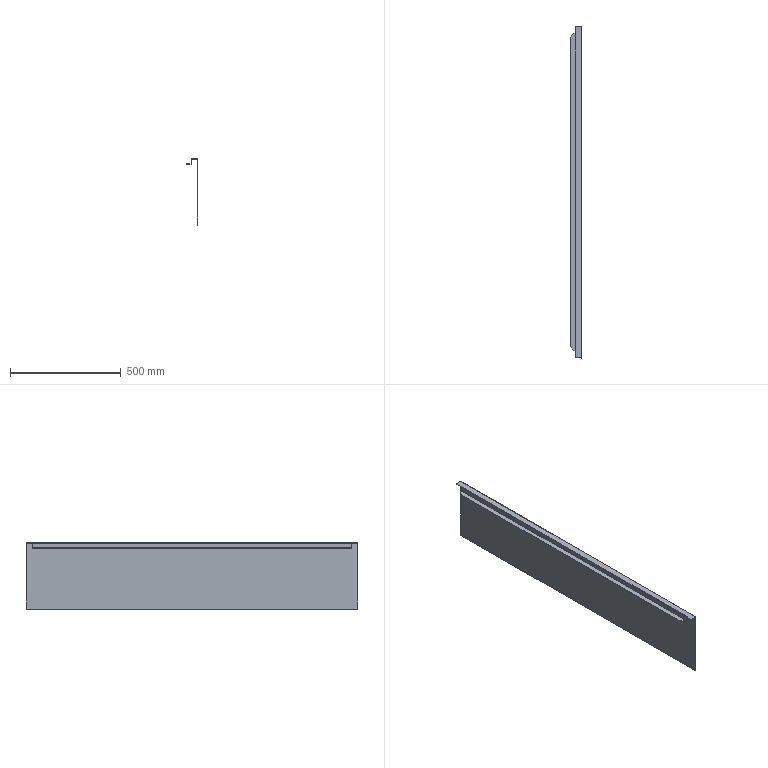Part | SolidWorks | features BaseBody 1, FlatPattern 1, FlattenBends 1, ProcessBends 1, SheetMetal 1 | 1 solid | 44 faces | box 52 x 1497 x 298.5 mm | volume 825530 mm3 | plane 36 | cylinder 6 | spline 2 | commonest cylinder face diameters 0.6 x3 3.6 x3
STEP:
#1=CARTESIAN_POINT('',(323.,-698.,276.5));
#2=VERTEX_POINT('',#1);
#3=CARTESIAN_POINT('',(323.,698.,276.5));
#4=VERTEX_POINT('',#3);
#5=CARTESIAN_POINT('',(323.,0.,276.5));
#6=DIRECTION('',(0.,1.,0.));
#7=VECTOR('',#6,1000.);
#8=LINE('',#5,#7);
#9=EDGE_CURVE('',#2,#4,#8,.T.);
#10=ORIENTED_EDGE('',*,*,#9,.F.);
#11=CARTESIAN_POINT('',(323.,-698.,278.));
#12=VERTEX_POINT('',#11);
#13=CARTESIAN_POINT('',(323.,-698.,3157.923));
#14=DIRECTION('',(0.,0.,-1.));
#15=VECTOR('',#14,1000.);
#16=LINE('',#13,#15);
#17=EDGE_CURVE('',#12,#2,#16,.T.);
#18=ORIENTED_EDGE('',*,*,#17,.F.);
#19=CARTESIAN_POINT('',(323.,698.,278.));
#20=VERTEX_POINT('',#19);
#21=CARTESIAN_POINT('',(323.,-698.,278.));
#22=DIRECTION('',(0.,1.,0.));
#23=VECTOR('',#22,1000.);
#24=LINE('',#21,#23);
#25=EDGE_CURVE('',#12,#20,#24,.T.);
#26=ORIENTED_EDGE('',*,*,#25,.T.);
#27=CARTESIAN_POINT('',(323.,698.,3157.923));
#28=DIRECTION('',(0.,0.,-1.));
#29=VECTOR('',#28,1000.);
#30=LINE('',#27,#29);
#31=EDGE_CURVE('',#20,#4,#30,.T.);
#32=ORIENTED_EDGE('',*,*,#31,.T.);
#33=EDGE_LOOP('',(#10,#18,#26,#32));
#34=FACE_OUTER_BOUND('',#33,.T.);
#35=CARTESIAN_POINT('',(323.,-698.,3157.923));
#36=DIRECTION('',(-1.,0.,0.));
#37=DIRECTION('',(0.,0.,1.));
#38=AXIS2_PLACEMENT_3D('',#35,#36,#37);
#39=PLANE('',#38);
#40=ADVANCED_FACE('',(#34),#39,.T.);
#41=CARTESIAN_POINT('',(344.7,719.899,276.5));
#42=VERTEX_POINT('',#41);
#43=CARTESIAN_POINT('',(-186.011,184.32,276.5));
#44=DIRECTION('',(0.7039,0.7103,0.));
#45=VECTOR('',#44,1000.);
#46=LINE('',#43,#45);
#47=EDGE_CURVE('',#4,#42,#46,.T.);
#48=ORIENTED_EDGE('',*,*,#47,.T.);
#49=CARTESIAN_POINT('',(344.7,-719.899,276.5));
#50=VERTEX_POINT('',#49);
#51=CARTESIAN_POINT('',(344.7,719.899,276.5));
#52=DIRECTION('',(0.,-1.,0.));
#53=VECTOR('',#52,1000.);
#54=LINE('',#51,#53);
#55=EDGE_CURVE('',#42,#50,#54,.T.);
#56=ORIENTED_EDGE('',*,*,#55,.T.);
#57=CARTESIAN_POINT('',(-186.011,-184.32,276.5));
#58=DIRECTION('',(0.7039,-0.7103,0.));
#59=VECTOR('',#58,1000.);
#60=LINE('',#57,#59);
#61=EDGE_CURVE('',#2,#50,#60,.T.);
#62=ORIENTED_EDGE('',*,*,#61,.F.);
#63=ORIENTED_EDGE('',*,*,#9,.T.);
#64=EDGE_LOOP('',(#48,#56,#62,#63));
#65=FACE_OUTER_BOUND('',#64,.T.);
#66=CARTESIAN_POINT('',(0.,0.,276.5));
#67=DIRECTION('',(0.,0.,1.));
#68=DIRECTION('',(1.,0.,0.));
#69=AXIS2_PLACEMENT_3D('',#66,#67,#68);
#70=PLANE('',#69);
#71=ADVANCED_FACE('',(#65),#70,.F.);
#72=ORIENTED_EDGE('',*,*,#17,.T.);
#73=ORIENTED_EDGE('',*,*,#61,.T.);
#74=CARTESIAN_POINT('',(344.7,-719.899,278.));
#75=VERTEX_POINT('',#74);
#76=CARTESIAN_POINT('',(344.7,-719.899,278.));
#77=CARTESIAN_POINT('',(344.7,-719.899,276.5));
#78=B_SPLINE_CURVE_WITH_KNOTS('',1,(#76,#77),.UNSPECIFIED.,.F.,.F.,(2,2),(0.,1.),.UNSPECIFIED.);
#79=EDGE_CURVE('',#75,#50,#78,.T.);
#80=ORIENTED_EDGE('',*,*,#79,.F.);
#81=CARTESIAN_POINT('',(-186.011,-184.32,278.));
#82=DIRECTION('',(0.7039,-0.7103,0.));
#83=VECTOR('',#82,1000.);
#84=LINE('',#81,#83);
#85=EDGE_CURVE('',#12,#75,#84,.T.);
#86=ORIENTED_EDGE('',*,*,#85,.F.);
#87=EDGE_LOOP('',(#72,#73,#80,#86));
#88=FACE_OUTER_BOUND('',#87,.T.);
#89=CARTESIAN_POINT('',(-186.011,-184.32,3157.923));
#90=DIRECTION('',(0.7103,0.7039,0.));
#91=DIRECTION('',(-0.7039,0.7103,0.));
#92=AXIS2_PLACEMENT_3D('',#89,#90,#91);
#93=PLANE('',#92);
#94=ADVANCED_FACE('',(#88),#93,.F.);
#95=CARTESIAN_POINT('',(344.7,719.899,278.));
#96=VERTEX_POINT('',#95);
#97=CARTESIAN_POINT('',(344.7,719.899,278.));
#98=DIRECTION('',(0.,-1.,0.));
#99=VECTOR('',#98,1000.);
#100=LINE('',#97,#99);
#101=EDGE_CURVE('',#96,#75,#100,.T.);
#102=ORIENTED_EDGE('',*,*,#101,.F.);
#103=CARTESIAN_POINT('',(-186.011,184.32,278.));
#104=DIRECTION('',(0.7039,0.7103,0.));
#105=VECTOR('',#104,1000.);
#106=LINE('',#103,#105);
#107=EDGE_CURVE('',#20,#96,#106,.T.);
#108=ORIENTED_EDGE('',*,*,#107,.F.);
#109=ORIENTED_EDGE('',*,*,#25,.F.);
#110=ORIENTED_EDGE('',*,*,#85,.T.);
#111=EDGE_LOOP('',(#102,#108,#109,#110));
#112=FACE_OUTER_BOUND('',#111,.T.);
#113=CARTESIAN_POINT('',(0.,0.,278.));
#114=DIRECTION('',(0.,0.,1.));
#115=DIRECTION('',(1.,0.,0.));
#116=AXIS2_PLACEMENT_3D('',#113,#114,#115);
#117=PLANE('',#116);
#118=ADVANCED_FACE('',(#112),#117,.T.);
#119=ORIENTED_EDGE('',*,*,#47,.F.);
#120=ORIENTED_EDGE('',*,*,#31,.F.);
#121=ORIENTED_EDGE('',*,*,#107,.T.);
#122=CARTESIAN_POINT('',(344.7,719.899,278.));
#123=CARTESIAN_POINT('',(344.7,719.899,277.5));
#124=CARTESIAN_POINT('',(344.7,719.899,277.));
#125=CARTESIAN_POINT('',(344.7,719.899,276.5));
#126=B_SPLINE_CURVE_WITH_KNOTS('',3,(#122,#123,#124,#125),.UNSPECIFIED.,.F.,.F.,(4,4),(0.,1.),.UNSPECIFIED.);
#127=EDGE_CURVE('',#96,#42,#126,.T.);
#128=ORIENTED_EDGE('',*,*,#127,.T.);
#129=EDGE_LOOP('',(#119,#120,#121,#128));
#130=FACE_OUTER_BOUND('',#129,.T.);
#131=CARTESIAN_POINT('',(-186.011,184.32,3157.923));
#132=DIRECTION('',(-0.7103,0.7039,0.));
#133=DIRECTION('',(-0.7039,-0.7103,0.));
#134=AXIS2_PLACEMENT_3D('',#131,#132,#133);
#135=PLANE('',#134);
#136=ADVANCED_FACE('',(#130),#135,.T.);
#137=CARTESIAN_POINT('',(346.5,720.,278.5));
#138=VERTEX_POINT('',#137);
#139=CARTESIAN_POINT('',(345.,720.,278.5));
#140=VERTEX_POINT('',#139);
#141=CARTESIAN_POINT('',(3231.274,720.,278.5));
#142=DIRECTION('',(-1.,0.,0.));
#143=VECTOR('',#142,1000.);
#144=LINE('',#141,#143);
#145=EDGE_CURVE('',#138,#140,#144,.T.);
#146=ORIENTED_EDGE('',*,*,#145,.T.);
#147=CARTESIAN_POINT('',(345.,721.5,278.5));
#148=VERTEX_POINT('',#147);
#149=CARTESIAN_POINT('',(345.,0.,278.5));
#150=DIRECTION('',(0.,-1.,0.));
#151=VECTOR('',#150,1000.);
#152=LINE('',#149,#151);
#153=EDGE_CURVE('',#148,#140,#152,.T.);
#154=ORIENTED_EDGE('',*,*,#153,.F.);
#155=CARTESIAN_POINT('',(346.5,721.5,278.5));
#156=VERTEX_POINT('',#155);
#157=CARTESIAN_POINT('',(3231.274,721.5,278.5));
#158=DIRECTION('',(-1.,0.,0.));
#159=VECTOR('',#158,1000.);
#160=LINE('',#157,#159);
#161=EDGE_CURVE('',#156,#148,#160,.T.);
#162=ORIENTED_EDGE('',*,*,#161,.F.);
#163=CARTESIAN_POINT('',(346.5,0.,278.5));
#164=DIRECTION('',(0.,1.,0.));
#165=VECTOR('',#164,1000.);
#166=LINE('',#163,#165);
#167=EDGE_CURVE('',#138,#156,#166,.T.);
#168=ORIENTED_EDGE('',*,*,#167,.F.);
#169=EDGE_LOOP('',(#146,#154,#162,#168));
#170=FACE_OUTER_BOUND('',#169,.T.);
#171=CARTESIAN_POINT('',(3231.274,0.,278.5));
#172=DIRECTION('',(0.,0.,1.));
#173=DIRECTION('',(1.,0.,0.));
#174=AXIS2_PLACEMENT_3D('',#171,#172,#173);
#175=PLANE('',#174);
#176=ADVANCED_FACE('',(#170),#175,.F.);
#177=CARTESIAN_POINT('',(345.,-720.,278.5));
#178=VERTEX_POINT('',#177);
#179=CARTESIAN_POINT('',(345.,-720.,278.3));
#180=VERTEX_POINT('',#179);
#181=CARTESIAN_POINT('',(345.,-720.,278.5));
#182=DIRECTION('',(0.,0.,-1.));
#183=VECTOR('',#182,1000.);
#184=LINE('',#181,#183);
#185=EDGE_CURVE('',#178,#180,#184,.T.);
#186=ORIENTED_EDGE('',*,*,#185,.T.);
#187=CARTESIAN_POINT('',(346.5,-720.,278.3));
#188=VERTEX_POINT('',#187);
#189=CARTESIAN_POINT('',(3231.274,-720.,278.3));
#190=DIRECTION('',(-1.,0.,0.));
#191=VECTOR('',#190,1000.);
#192=LINE('',#189,#191);
#193=EDGE_CURVE('',#188,#180,#192,.T.);
#194=ORIENTED_EDGE('',*,*,#193,.F.);
#195=CARTESIAN_POINT('',(346.5,-720.,278.5));
#196=VERTEX_POINT('',#195);
#197=CARTESIAN_POINT('',(346.5,-720.,278.));
#198=DIRECTION('',(0.,0.,1.));
#199=VECTOR('',#198,1000.);
#200=LINE('',#197,#199);
#201=EDGE_CURVE('',#188,#196,#200,.T.);
#202=ORIENTED_EDGE('',*,*,#201,.T.);
#203=CARTESIAN_POINT('',(3231.274,-720.,278.5));
#204=DIRECTION('',(-1.,0.,0.));
#205=VECTOR('',#204,1000.);
#206=LINE('',#203,#205);
#207=EDGE_CURVE('',#196,#178,#206,.T.);
#208=ORIENTED_EDGE('',*,*,#207,.T.);
#209=EDGE_LOOP('',(#186,#194,#202,#208));
#210=FACE_OUTER_BOUND('',#209,.T.);
#211=CARTESIAN_POINT('',(3231.274,-720.,278.));
#212=DIRECTION('',(0.,-1.,0.));
#213=DIRECTION('',(0.,0.,1.));
#214=AXIS2_PLACEMENT_3D('',#211,#212,#213);
#215=PLANE('',#214);
#216=ADVANCED_FACE('',(#210),#215,.T.);
#217=CARTESIAN_POINT('',(345.,720.,278.3));
#218=VERTEX_POINT('',#217);
#219=CARTESIAN_POINT('',(345.,720.,278.5));
#220=DIRECTION('',(0.,0.,1.));
#221=VECTOR('',#220,1000.);
#222=LINE('',#219,#221);
#223=EDGE_CURVE('',#218,#140,#222,.T.);
#224=ORIENTED_EDGE('',*,*,#223,.T.);
#225=ORIENTED_EDGE('',*,*,#145,.F.);
#226=CARTESIAN_POINT('',(346.5,720.,278.3));
#227=VERTEX_POINT('',#226);
#228=CARTESIAN_POINT('',(346.5,720.,278.));
#229=DIRECTION('',(0.,0.,-1.));
#230=VECTOR('',#229,1000.);
#231=LINE('',#228,#230);
#232=EDGE_CURVE('',#138,#227,#231,.T.);
#233=ORIENTED_EDGE('',*,*,#232,.T.);
#234=CARTESIAN_POINT('',(3231.274,720.,278.3));
#235=DIRECTION('',(-1.,0.,0.));
#236=VECTOR('',#235,1000.);
#237=LINE('',#234,#236);
#238=EDGE_CURVE('',#227,#218,#237,.T.);
#239=ORIENTED_EDGE('',*,*,#238,.T.);
#240=EDGE_LOOP('',(#224,#225,#233,#239));
#241=FACE_OUTER_BOUND('',#240,.T.);
#242=CARTESIAN_POINT('',(3231.274,720.,278.));
#243=DIRECTION('',(0.,1.,0.));
#244=DIRECTION('',(0.,0.,-1.));
#245=AXIS2_PLACEMENT_3D('',#242,#243,#244);
#246=PLANE('',#245);
#247=ADVANCED_FACE('',(#241),#246,.T.);
#248=CARTESIAN_POINT('',(346.5,-721.5,278.5));
#249=VERTEX_POINT('',#248);
#250=CARTESIAN_POINT('',(345.,-721.5,278.5));
#251=VERTEX_POINT('',#250);
#252=CARTESIAN_POINT('',(3231.274,-721.5,278.5));
#253=DIRECTION('',(-1.,0.,0.));
#254=VECTOR('',#253,1000.);
#255=LINE('',#252,#254);
#256=EDGE_CURVE('',#249,#251,#255,.T.);
#257=ORIENTED_EDGE('',*,*,#256,.T.);
#258=CARTESIAN_POINT('',(345.,0.,278.5));
#259=DIRECTION('',(0.,-1.,0.));
#260=VECTOR('',#259,1000.);
#261=LINE('',#258,#260);
#262=EDGE_CURVE('',#178,#251,#261,.T.);
#263=ORIENTED_EDGE('',*,*,#262,.F.);
#264=ORIENTED_EDGE('',*,*,#207,.F.);
#265=CARTESIAN_POINT('',(346.5,0.,278.5));
#266=DIRECTION('',(0.,1.,0.));
#267=VECTOR('',#266,1000.);
#268=LINE('',#265,#267);
#269=EDGE_CURVE('',#249,#196,#268,.T.);
#270=ORIENTED_EDGE('',*,*,#269,.F.);
#271=EDGE_LOOP('',(#257,#263,#264,#270));
#272=FACE_OUTER_BOUND('',#271,.T.);
#273=CARTESIAN_POINT('',(3231.274,0.,278.5));
#274=DIRECTION('',(0.,0.,1.));
#275=DIRECTION('',(1.,0.,0.));
#276=AXIS2_PLACEMENT_3D('',#273,#274,#275);
#277=PLANE('',#276);
#278=ADVANCED_FACE('',(#272),#277,.F.);
#279=CARTESIAN_POINT('',(345.,-721.5,298.2));
#280=VERTEX_POINT('',#279);
#281=CARTESIAN_POINT('',(345.,-721.5,278.));
#282=DIRECTION('',(0.,0.,-1.));
#283=VECTOR('',#282,1000.);
#284=LINE('',#281,#283);
#285=EDGE_CURVE('',#280,#251,#284,.T.);
#286=ORIENTED_EDGE('',*,*,#285,.T.);
#287=ORIENTED_EDGE('',*,*,#256,.F.);
#288=CARTESIAN_POINT('',(346.5,-721.5,298.2));
#289=VERTEX_POINT('',#288);
#290=CARTESIAN_POINT('',(346.5,-721.5,278.));
#291=DIRECTION('',(0.,0.,1.));
#292=VECTOR('',#291,1000.);
#293=LINE('',#290,#292);
#294=EDGE_CURVE('',#249,#289,#293,.T.);
#295=ORIENTED_EDGE('',*,*,#294,.T.);
#296=CARTESIAN_POINT('',(3231.274,-721.5,298.2));
#297=DIRECTION('',(-1.,0.,0.));
#298=VECTOR('',#297,1000.);
#299=LINE('',#296,#298);
#300=EDGE_CURVE('',#289,#280,#299,.T.);
#301=ORIENTED_EDGE('',*,*,#300,.T.);
#302=EDGE_LOOP('',(#286,#287,#295,#301));
#303=FACE_OUTER_BOUND('',#302,.T.);
#304=CARTESIAN_POINT('',(3231.274,-721.5,278.));
#305=DIRECTION('',(0.,-1.,0.));
#306=DIRECTION('',(0.,0.,1.));
#307=AXIS2_PLACEMENT_3D('',#304,#305,#306);
#308=PLANE('',#307);
#309=ADVANCED_FACE('',(#303),#308,.T.);
#310=ORIENTED_EDGE('',*,*,#223,.F.);
#311=CARTESIAN_POINT('',(345.,720.,278.3));
#312=DIRECTION('',(0.,-1.,0.));
#313=VECTOR('',#312,1000.);
#314=LINE('',#311,#313);
#315=EDGE_CURVE('',#218,#180,#314,.T.);
#316=ORIENTED_EDGE('',*,*,#315,.T.);
#317=ORIENTED_EDGE('',*,*,#185,.F.);
#318=ORIENTED_EDGE('',*,*,#262,.T.);
#319=ORIENTED_EDGE('',*,*,#285,.F.);
#320=CARTESIAN_POINT('',(345.,721.5,298.2));
#321=VERTEX_POINT('',#320);
#322=CARTESIAN_POINT('',(345.,-721.5,298.2));
#323=DIRECTION('',(0.,1.,0.));
#324=VECTOR('',#323,1000.);
#325=LINE('',#322,#324);
#326=EDGE_CURVE('',#280,#321,#325,.T.);
#327=ORIENTED_EDGE('',*,*,#326,.T.);
#328=CARTESIAN_POINT('',(345.,721.5,278.));
#329=DIRECTION('',(0.,0.,1.));
#330=VECTOR('',#329,1000.);
#331=LINE('',#328,#330);
#332=EDGE_CURVE('',#148,#321,#331,.T.);
#333=ORIENTED_EDGE('',*,*,#332,.F.);
#334=ORIENTED_EDGE('',*,*,#153,.T.);
#335=EDGE_LOOP('',(#310,#316,#317,#318,#319,#327,#333,#334));
#336=FACE_OUTER_BOUND('',#335,.T.);
#337=CARTESIAN_POINT('',(345.,-720.,278.));
#338=DIRECTION('',(1.,0.,0.));
#339=DIRECTION('',(0.,1.,0.));
#340=AXIS2_PLACEMENT_3D('',#337,#338,#339);
#341=PLANE('',#340);
#342=ADVANCED_FACE('',(#336),#341,.F.);
#343=ORIENTED_EDGE('',*,*,#161,.T.);
#344=ORIENTED_EDGE('',*,*,#332,.T.);
#345=CARTESIAN_POINT('',(346.5,721.5,298.2));
#346=VERTEX_POINT('',#345);
#347=CARTESIAN_POINT('',(3231.274,721.5,298.2));
#348=DIRECTION('',(-1.,0.,0.));
#349=VECTOR('',#348,1000.);
#350=LINE('',#347,#349);
#351=EDGE_CURVE('',#346,#321,#350,.T.);
#352=ORIENTED_EDGE('',*,*,#351,.F.);
#353=CARTESIAN_POINT('',(346.5,721.5,278.));
#354=DIRECTION('',(0.,0.,1.));
#355=VECTOR('',#354,1000.);
#356=LINE('',#353,#355);
#357=EDGE_CURVE('',#156,#346,#356,.T.);
#358=ORIENTED_EDGE('',*,*,#357,.F.);
#359=EDGE_LOOP('',(#343,#344,#352,#358));
#360=FACE_OUTER_BOUND('',#359,.T.);
#361=CARTESIAN_POINT('',(3231.274,721.5,278.));
#362=DIRECTION('',(0.,-1.,0.));
#363=DIRECTION('',(0.,0.,1.));
#364=AXIS2_PLACEMENT_3D('',#361,#362,#363);
#365=PLANE('',#364);
#366=ADVANCED_FACE('',(#360),#365,.F.);
#367=CARTESIAN_POINT('',(346.5,720.,278.3));
#368=DIRECTION('',(0.,-1.,0.));
#369=VECTOR('',#368,1000.);
#370=LINE('',#367,#369);
#371=EDGE_CURVE('',#227,#188,#370,.T.);
#372=ORIENTED_EDGE('',*,*,#371,.F.);
#373=ORIENTED_EDGE('',*,*,#232,.F.);
#374=ORIENTED_EDGE('',*,*,#167,.T.);
#375=ORIENTED_EDGE('',*,*,#357,.T.);
#376=CARTESIAN_POINT('',(346.5,-721.5,298.2));
#377=DIRECTION('',(0.,1.,0.));
#378=VECTOR('',#377,1000.);
#379=LINE('',#376,#378);
#380=EDGE_CURVE('',#289,#346,#379,.T.);
#381=ORIENTED_EDGE('',*,*,#380,.F.);
#382=ORIENTED_EDGE('',*,*,#294,.F.);
#383=ORIENTED_EDGE('',*,*,#269,.T.);
#384=ORIENTED_EDGE('',*,*,#201,.F.);
#385=EDGE_LOOP('',(#372,#373,#374,#375,#381,#382,#383,#384));
#386=FACE_OUTER_BOUND('',#385,.T.);
#387=CARTESIAN_POINT('',(346.5,-720.,278.));
#388=DIRECTION('',(1.,0.,0.));
#389=DIRECTION('',(0.,1.,0.));
#390=AXIS2_PLACEMENT_3D('',#387,#388,#389);
#391=PLANE('',#390);
#392=ADVANCED_FACE('',(#386),#391,.T.);
#393=CARTESIAN_POINT('',(346.8,-721.5,298.5));
#394=VERTEX_POINT('',#393);
#395=CARTESIAN_POINT('',(347.,-721.5,298.5));
#396=VERTEX_POINT('',#395);
#397=CARTESIAN_POINT('',(344.5,-721.5,298.5));
#398=DIRECTION('',(1.,0.,0.));
#399=VECTOR('',#398,1000.);
#400=LINE('',#397,#399);
#401=EDGE_CURVE('',#394,#396,#400,.T.);
#402=ORIENTED_EDGE('',*,*,#401,.F.);
#403=CARTESIAN_POINT('',(346.8,721.5,298.5));
#404=VERTEX_POINT('',#403);
#405=CARTESIAN_POINT('',(346.8,-721.5,298.5));
#406=DIRECTION('',(0.,1.,0.));
#407=VECTOR('',#406,1000.);
#408=LINE('',#405,#407);
#409=EDGE_CURVE('',#394,#404,#408,.T.);
#410=ORIENTED_EDGE('',*,*,#409,.T.);
#411=CARTESIAN_POINT('',(347.,721.5,298.5));
#412=VERTEX_POINT('',#411);
#413=CARTESIAN_POINT('',(347.,721.5,298.5));
#414=DIRECTION('',(-1.,0.,0.));
#415=VECTOR('',#414,1000.);
#416=LINE('',#413,#415);
#417=EDGE_CURVE('',#412,#404,#416,.T.);
#418=ORIENTED_EDGE('',*,*,#417,.F.);
#419=CARTESIAN_POINT('',(347.,721.9,298.5));
#420=VERTEX_POINT('',#419);
#421=CARTESIAN_POINT('',(347.,721.5,298.5));
#422=DIRECTION('',(0.,-1.,0.));
#423=VECTOR('',#422,1000.);
#424=LINE('',#421,#423);
#425=EDGE_CURVE('',#420,#412,#424,.T.);
#426=ORIENTED_EDGE('',*,*,#425,.F.);
#427=CARTESIAN_POINT('',(345.,721.9,298.5));
#428=VERTEX_POINT('',#427);
#429=CARTESIAN_POINT('',(347.,721.9,298.5));
#430=DIRECTION('',(1.,0.,0.));
#431=VECTOR('',#430,1000.);
#432=LINE('',#429,#431);
#433=EDGE_CURVE('',#428,#420,#432,.T.);
#434=ORIENTED_EDGE('',*,*,#433,.F.);
#435=CARTESIAN_POINT('',(345.,748.3,298.5));
#436=VERTEX_POINT('',#435);
#437=CARTESIAN_POINT('',(345.,0.,298.5));
#438=DIRECTION('',(0.,1.,0.));
#439=VECTOR('',#438,1000.);
#440=LINE('',#437,#439);
#441=EDGE_CURVE('',#428,#436,#440,.T.);
#442=ORIENTED_EDGE('',*,*,#441,.T.);
#443=CARTESIAN_POINT('',(373.2,748.3,298.5));
#444=VERTEX_POINT('',#443);
#445=CARTESIAN_POINT('',(0.,748.3,298.5));
#446=DIRECTION('',(1.,0.,0.));
#447=VECTOR('',#446,1000.);
#448=LINE('',#445,#447);
#449=EDGE_CURVE('',#436,#444,#448,.T.);
#450=ORIENTED_EDGE('',*,*,#449,.T.);
#451=CARTESIAN_POINT('',(373.2,-748.3,298.5));
#452=VERTEX_POINT('',#451);
#453=CARTESIAN_POINT('',(373.2,-748.3,298.5));
#454=DIRECTION('',(0.,1.,0.));
#455=VECTOR('',#454,1000.);
#456=LINE('',#453,#455);
#457=EDGE_CURVE('',#452,#444,#456,.T.);
#458=ORIENTED_EDGE('',*,*,#457,.F.);
#459=CARTESIAN_POINT('',(345.,-748.3,298.5));
#460=VERTEX_POINT('',#459);
#461=CARTESIAN_POINT('',(0.,-748.3,298.5));
#462=DIRECTION('',(-1.,0.,0.));
#463=VECTOR('',#462,1000.);
#464=LINE('',#461,#463);
#465=EDGE_CURVE('',#452,#460,#464,.T.);
#466=ORIENTED_EDGE('',*,*,#465,.T.);
#467=CARTESIAN_POINT('',(345.,-721.9,298.5));
#468=VERTEX_POINT('',#467);
#469=CARTESIAN_POINT('',(345.,0.,298.5));
#470=DIRECTION('',(0.,1.,0.));
#471=VECTOR('',#470,1000.);
#472=LINE('',#469,#471);
#473=EDGE_CURVE('',#460,#468,#472,.T.);
#474=ORIENTED_EDGE('',*,*,#473,.T.);
#475=CARTESIAN_POINT('',(347.,-721.9,298.5));
#476=VERTEX_POINT('',#475);
#477=CARTESIAN_POINT('',(344.5,-721.9,298.5));
#478=DIRECTION('',(-1.,0.,0.));
#479=VECTOR('',#478,1000.);
#480=LINE('',#477,#479);
#481=EDGE_CURVE('',#476,#468,#480,.T.);
#482=ORIENTED_EDGE('',*,*,#481,.F.);
#483=CARTESIAN_POINT('',(347.,-721.5,298.5));
#484=DIRECTION('',(0.,-1.,0.));
#485=VECTOR('',#484,1000.);
#486=LINE('',#483,#485);
#487=EDGE_CURVE('',#396,#476,#486,.T.);
#488=ORIENTED_EDGE('',*,*,#487,.F.);
#489=EDGE_LOOP('',(#402,#410,#418,#426,#434,#442,#450,#458,#466,#474,#482,#488));
#490=FACE_OUTER_BOUND('',#489,.T.);
#491=CARTESIAN_POINT('',(0.,0.,298.5));
#492=DIRECTION('',(0.,0.,-1.));
#493=DIRECTION('',(-1.,0.,0.));
#494=AXIS2_PLACEMENT_3D('',#491,#492,#493);
#495=PLANE('',#494);
#496=ADVANCED_FACE('',(#490),#495,.T.);
#497=CARTESIAN_POINT('',(346.8,-721.5,300.));
#498=VERTEX_POINT('',#497);
#499=CARTESIAN_POINT('',(347.,-721.5,300.));
#500=VERTEX_POINT('',#499);
#501=CARTESIAN_POINT('',(0.,-721.5,300.));
#502=DIRECTION('',(1.,0.,0.));
#503=VECTOR('',#502,1000.);
#504=LINE('',#501,#503);
#505=EDGE_CURVE('',#498,#500,#504,.T.);
#506=ORIENTED_EDGE('',*,*,#505,.F.);
#507=CARTESIAN_POINT('',(346.8,-721.5,-2693.731));
#508=DIRECTION('',(0.,0.,1.));
#509=VECTOR('',#508,1000.);
#510=LINE('',#507,#509);
#511=EDGE_CURVE('',#394,#498,#510,.T.);
#512=ORIENTED_EDGE('',*,*,#511,.F.);
#513=ORIENTED_EDGE('',*,*,#401,.T.);
#514=CARTESIAN_POINT('',(347.,-721.5,-2693.731));
#515=DIRECTION('',(0.,0.,1.));
#516=VECTOR('',#515,1000.);
#517=LINE('',#514,#516);
#518=EDGE_CURVE('',#396,#500,#517,.T.);
#519=ORIENTED_EDGE('',*,*,#518,.T.);
#520=EDGE_LOOP('',(#506,#512,#513,#519));
#521=FACE_OUTER_BOUND('',#520,.T.);
#522=CARTESIAN_POINT('',(344.5,-721.5,-2693.731));
#523=DIRECTION('',(0.,-1.,0.));
#524=DIRECTION('',(0.,0.,1.));
#525=AXIS2_PLACEMENT_3D('',#522,#523,#524);
#526=PLANE('',#525);
#527=ADVANCED_FACE('',(#521),#526,.T.);
#528=CARTESIAN_POINT('',(347.,721.5,300.));
#529=VERTEX_POINT('',#528);
#530=CARTESIAN_POINT('',(346.8,721.5,300.));
#531=VERTEX_POINT('',#530);
#532=CARTESIAN_POINT('',(0.,721.5,300.));
#533=DIRECTION('',(-1.,0.,0.));
#534=VECTOR('',#533,1000.);
#535=LINE('',#532,#534);
#536=EDGE_CURVE('',#529,#531,#535,.T.);
#537=ORIENTED_EDGE('',*,*,#536,.F.);
#538=CARTESIAN_POINT('',(347.,721.5,-2693.731));
#539=DIRECTION('',(0.,0.,1.));
#540=VECTOR('',#539,1000.);
#541=LINE('',#538,#540);
#542=EDGE_CURVE('',#412,#529,#541,.T.);
#543=ORIENTED_EDGE('',*,*,#542,.F.);
#544=ORIENTED_EDGE('',*,*,#417,.T.);
#545=CARTESIAN_POINT('',(346.8,721.5,-2693.731));
#546=DIRECTION('',(0.,0.,1.));
#547=VECTOR('',#546,1000.);
#548=LINE('',#545,#547);
#549=EDGE_CURVE('',#404,#531,#548,.T.);
#550=ORIENTED_EDGE('',*,*,#549,.T.);
#551=EDGE_LOOP('',(#537,#543,#544,#550));
#552=FACE_OUTER_BOUND('',#551,.T.);
#553=CARTESIAN_POINT('',(347.,721.5,-2693.731));
#554=DIRECTION('',(0.,1.,0.));
#555=DIRECTION('',(0.,0.,-1.));
#556=AXIS2_PLACEMENT_3D('',#553,#554,#555);
#557=PLANE('',#556);
#558=ADVANCED_FACE('',(#552),#557,.T.);
#559=CARTESIAN_POINT('',(347.,721.9,300.));
#560=VERTEX_POINT('',#559);
#561=CARTESIAN_POINT('',(347.,0.,300.));
#562=DIRECTION('',(0.,-1.,0.));
#563=VECTOR('',#562,1000.);
#564=LINE('',#561,#563);
#565=EDGE_CURVE('',#560,#529,#564,.T.);
#566=ORIENTED_EDGE('',*,*,#565,.F.);
#567=CARTESIAN_POINT('',(347.,721.9,-2693.731));
#568=DIRECTION('',(0.,0.,1.));
#569=VECTOR('',#568,1000.);
#570=LINE('',#567,#569);
#571=EDGE_CURVE('',#420,#560,#570,.T.);
#572=ORIENTED_EDGE('',*,*,#571,.F.);
#573=ORIENTED_EDGE('',*,*,#425,.T.);
#574=ORIENTED_EDGE('',*,*,#542,.T.);
#575=EDGE_LOOP('',(#566,#572,#573,#574));
#576=FACE_OUTER_BOUND('',#575,.T.);
#577=CARTESIAN_POINT('',(347.,721.5,-2693.731));
#578=DIRECTION('',(-1.,0.,0.));
#579=DIRECTION('',(0.,0.,1.));
#580=AXIS2_PLACEMENT_3D('',#577,#578,#579);
#581=PLANE('',#580);
#582=ADVANCED_FACE('',(#576),#581,.T.);
#583=CARTESIAN_POINT('',(345.,721.9,300.));
#584=VERTEX_POINT('',#583);
#585=CARTESIAN_POINT('',(0.,721.9,300.));
#586=DIRECTION('',(1.,0.,0.));
#587=VECTOR('',#586,1000.);
#588=LINE('',#585,#587);
#589=EDGE_CURVE('',#584,#560,#588,.T.);
#590=ORIENTED_EDGE('',*,*,#589,.F.);
#591=CARTESIAN_POINT('',(345.,721.9,-2693.731));
#592=DIRECTION('',(0.,0.,1.));
#593=VECTOR('',#592,1000.);
#594=LINE('',#591,#593);
#595=EDGE_CURVE('',#428,#584,#594,.T.);
#596=ORIENTED_EDGE('',*,*,#595,.F.);
#597=ORIENTED_EDGE('',*,*,#433,.T.);
#598=ORIENTED_EDGE('',*,*,#571,.T.);
#599=EDGE_LOOP('',(#590,#596,#597,#598));
#600=FACE_OUTER_BOUND('',#599,.T.);
#601=CARTESIAN_POINT('',(347.,721.9,-2693.731));
#602=DIRECTION('',(0.,-1.,0.));
#603=DIRECTION('',(0.,0.,1.));
#604=AXIS2_PLACEMENT_3D('',#601,#602,#603);
#605=PLANE('',#604);
#606=ADVANCED_FACE('',(#600),#605,.T.);
#607=ORIENTED_EDGE('',*,*,#595,.T.);
#608=CARTESIAN_POINT('',(345.,748.3,300.));
#609=VERTEX_POINT('',#608);
#610=CARTESIAN_POINT('',(345.,-720.,300.));
#611=DIRECTION('',(0.,1.,0.));
#612=VECTOR('',#611,1000.);
#613=LINE('',#610,#612);
#614=EDGE_CURVE('',#584,#609,#613,.T.);
#615=ORIENTED_EDGE('',*,*,#614,.T.);
#616=CARTESIAN_POINT('',(345.,748.3,-2693.731));
#617=DIRECTION('',(0.,0.,1.));
#618=VECTOR('',#617,1000.);
#619=LINE('',#616,#618);
#620=EDGE_CURVE('',#436,#609,#619,.T.);
#621=ORIENTED_EDGE('',*,*,#620,.F.);
#622=ORIENTED_EDGE('',*,*,#441,.F.);
#623=EDGE_LOOP('',(#607,#615,#621,#622));
#624=FACE_OUTER_BOUND('',#623,.T.);
#625=CARTESIAN_POINT('',(345.,0.,-2693.731));
#626=DIRECTION('',(1.,0.,0.));
#627=DIRECTION('',(0.,0.,-1.));
#628=AXIS2_PLACEMENT_3D('',#625,#626,#627);
#629=PLANE('',#628);
#630=ADVANCED_FACE('',(#624),#629,.F.);
#631=ORIENTED_EDGE('',*,*,#620,.T.);
#632=CARTESIAN_POINT('',(373.2,748.3,300.));
#633=VERTEX_POINT('',#632);
#634=CARTESIAN_POINT('',(345.,748.3,300.));
#635=DIRECTION('',(1.,0.,0.));
#636=VECTOR('',#635,1000.);
#637=LINE('',#634,#636);
#638=EDGE_CURVE('',#609,#633,#637,.T.);
#639=ORIENTED_EDGE('',*,*,#638,.T.);
#640=CARTESIAN_POINT('',(373.2,748.3,-2693.731));
#641=DIRECTION('',(0.,0.,1.));
#642=VECTOR('',#641,1000.);
#643=LINE('',#640,#642);
#644=EDGE_CURVE('',#444,#633,#643,.T.);
#645=ORIENTED_EDGE('',*,*,#644,.F.);
#646=ORIENTED_EDGE('',*,*,#449,.F.);
#647=EDGE_LOOP('',(#631,#639,#645,#646));
#648=FACE_OUTER_BOUND('',#647,.T.);
#649=CARTESIAN_POINT('',(0.,748.3,-2693.731));
#650=DIRECTION('',(0.,-1.,0.));
#651=DIRECTION('',(0.,0.,1.));
#652=AXIS2_PLACEMENT_3D('',#649,#650,#651);
#653=PLANE('',#652);
#654=ADVANCED_FACE('',(#648),#653,.F.);
#655=CARTESIAN_POINT('',(373.2,-748.3,300.));
#656=VERTEX_POINT('',#655);
#657=CARTESIAN_POINT('',(373.2,-748.3,-2693.731));
#658=DIRECTION('',(0.,0.,1.));
#659=VECTOR('',#658,1000.);
#660=LINE('',#657,#659);
#661=EDGE_CURVE('',#452,#656,#660,.T.);
#662=ORIENTED_EDGE('',*,*,#661,.T.);
#663=CARTESIAN_POINT('',(345.,-748.3,300.));
#664=VERTEX_POINT('',#663);
#665=CARTESIAN_POINT('',(345.,-748.3,300.));
#666=DIRECTION('',(-1.,0.,0.));
#667=VECTOR('',#666,1000.);
#668=LINE('',#665,#667);
#669=EDGE_CURVE('',#656,#664,#668,.T.);
#670=ORIENTED_EDGE('',*,*,#669,.T.);
#671=CARTESIAN_POINT('',(345.,-748.3,-2693.731));
#672=DIRECTION('',(0.,0.,1.));
#673=VECTOR('',#672,1000.);
#674=LINE('',#671,#673);
#675=EDGE_CURVE('',#460,#664,#674,.T.);
#676=ORIENTED_EDGE('',*,*,#675,.F.);
#677=ORIENTED_EDGE('',*,*,#465,.F.);
#678=EDGE_LOOP('',(#662,#670,#676,#677));
#679=FACE_OUTER_BOUND('',#678,.T.);
#680=CARTESIAN_POINT('',(0.,-748.3,-2693.731));
#681=DIRECTION('',(0.,1.,0.));
#682=DIRECTION('',(0.,0.,-1.));
#683=AXIS2_PLACEMENT_3D('',#680,#681,#682);
#684=PLANE('',#683);
#685=ADVANCED_FACE('',(#679),#684,.F.);
#686=ORIENTED_EDGE('',*,*,#675,.T.);
#687=CARTESIAN_POINT('',(345.,-721.9,300.));
#688=VERTEX_POINT('',#687);
#689=CARTESIAN_POINT('',(345.,-720.,300.));
#690=DIRECTION('',(0.,1.,0.));
#691=VECTOR('',#690,1000.);
#692=LINE('',#689,#691);
#693=EDGE_CURVE('',#664,#688,#692,.T.);
#694=ORIENTED_EDGE('',*,*,#693,.T.);
#695=CARTESIAN_POINT('',(345.,-721.9,-2693.731));
#696=DIRECTION('',(0.,0.,1.));
#697=VECTOR('',#696,1000.);
#698=LINE('',#695,#697);
#699=EDGE_CURVE('',#468,#688,#698,.T.);
#700=ORIENTED_EDGE('',*,*,#699,.F.);
#701=ORIENTED_EDGE('',*,*,#473,.F.);
#702=EDGE_LOOP('',(#686,#694,#700,#701));
#703=FACE_OUTER_BOUND('',#702,.T.);
#704=CARTESIAN_POINT('',(345.,0.,-2693.731));
#705=DIRECTION('',(1.,0.,0.));
#706=DIRECTION('',(0.,0.,-1.));
#707=AXIS2_PLACEMENT_3D('',#704,#705,#706);
#708=PLANE('',#707);
#709=ADVANCED_FACE('',(#703),#708,.F.);
#710=CARTESIAN_POINT('',(347.,-721.9,300.));
#711=VERTEX_POINT('',#710);
#712=CARTESIAN_POINT('',(0.,-721.9,300.));
#713=DIRECTION('',(-1.,0.,0.));
#714=VECTOR('',#713,1000.);
#715=LINE('',#712,#714);
#716=EDGE_CURVE('',#711,#688,#715,.T.);
#717=ORIENTED_EDGE('',*,*,#716,.F.);
#718=CARTESIAN_POINT('',(347.,-721.9,-2693.731));
#719=DIRECTION('',(0.,0.,1.));
#720=VECTOR('',#719,1000.);
#721=LINE('',#718,#720);
#722=EDGE_CURVE('',#476,#711,#721,.T.);
#723=ORIENTED_EDGE('',*,*,#722,.F.);
#724=ORIENTED_EDGE('',*,*,#481,.T.);
#725=ORIENTED_EDGE('',*,*,#699,.T.);
#726=EDGE_LOOP('',(#717,#723,#724,#725));
#727=FACE_OUTER_BOUND('',#726,.T.);
#728=CARTESIAN_POINT('',(344.5,-721.9,-2693.731));
#729=DIRECTION('',(0.,1.,0.));
#730=DIRECTION('',(0.,0.,-1.));
#731=AXIS2_PLACEMENT_3D('',#728,#729,#730);
#732=PLANE('',#731);
#733=ADVANCED_FACE('',(#727),#732,.T.);
#734=CARTESIAN_POINT('',(347.,0.,300.));
#735=DIRECTION('',(0.,-1.,0.));
#736=VECTOR('',#735,1000.);
#737=LINE('',#734,#736);
#738=EDGE_CURVE('',#500,#711,#737,.T.);
#739=ORIENTED_EDGE('',*,*,#738,.F.);
#740=ORIENTED_EDGE('',*,*,#518,.F.);
#741=ORIENTED_EDGE('',*,*,#487,.T.);
#742=ORIENTED_EDGE('',*,*,#722,.T.);
#743=EDGE_LOOP('',(#739,#740,#741,#742));
#744=FACE_OUTER_BOUND('',#743,.T.);
#745=CARTESIAN_POINT('',(347.,-721.5,-2693.731));
#746=DIRECTION('',(-1.,0.,0.));
#747=DIRECTION('',(0.,0.,1.));
#748=AXIS2_PLACEMENT_3D('',#745,#746,#747);
#749=PLANE('',#748);
#750=ADVANCED_FACE('',(#744),#749,.T.);
#751=CARTESIAN_POINT('',(346.8,-721.5,300.));
#752=DIRECTION('',(0.,1.,0.));
#753=VECTOR('',#752,1000.);
#754=LINE('',#751,#753);
#755=EDGE_CURVE('',#498,#531,#754,.T.);
#756=ORIENTED_EDGE('',*,*,#755,.F.);
#757=ORIENTED_EDGE('',*,*,#505,.T.);
#758=ORIENTED_EDGE('',*,*,#738,.T.);
#759=ORIENTED_EDGE('',*,*,#716,.T.);
#760=ORIENTED_EDGE('',*,*,#693,.F.);
#761=ORIENTED_EDGE('',*,*,#669,.F.);
#762=CARTESIAN_POINT('',(373.2,-748.3,300.));
#763=DIRECTION('',(0.,1.,0.));
#764=VECTOR('',#763,1000.);
#765=LINE('',#762,#764);
#766=EDGE_CURVE('',#656,#633,#765,.T.);
#767=ORIENTED_EDGE('',*,*,#766,.T.);
#768=ORIENTED_EDGE('',*,*,#638,.F.);
#769=ORIENTED_EDGE('',*,*,#614,.F.);
#770=ORIENTED_EDGE('',*,*,#589,.T.);
#771=ORIENTED_EDGE('',*,*,#565,.T.);
#772=ORIENTED_EDGE('',*,*,#536,.T.);
#773=EDGE_LOOP('',(#756,#757,#758,#759,#760,#761,#767,#768,#769,#770,#771,#772));
#774=FACE_OUTER_BOUND('',#773,.T.);
#775=CARTESIAN_POINT('',(0.,0.,300.));
#776=DIRECTION('',(0.,0.,-1.));
#777=DIRECTION('',(-1.,0.,0.));
#778=AXIS2_PLACEMENT_3D('',#775,#776,#777);
#779=PLANE('',#778);
#780=ADVANCED_FACE('',(#774),#779,.F.);
#781=CARTESIAN_POINT('',(375.,-748.3,1.5));
#782=VERTEX_POINT('',#781);
#783=CARTESIAN_POINT('',(375.,748.3,1.5));
#784=VERTEX_POINT('',#783);
#785=CARTESIAN_POINT('',(375.,-750.,1.5));
#786=DIRECTION('',(0.,1.,0.));
#787=VECTOR('',#786,1000.);
#788=LINE('',#785,#787);
#789=EDGE_CURVE('',#782,#784,#788,.T.);
#790=ORIENTED_EDGE('',*,*,#789,.F.);
#791=CARTESIAN_POINT('',(373.5,-748.3,1.5));
#792=VERTEX_POINT('',#791);
#793=CARTESIAN_POINT('',(-2676.454,-748.3,1.5));
#794=DIRECTION('',(1.,0.,0.));
#795=VECTOR('',#794,1000.);
#796=LINE('',#793,#795);
#797=EDGE_CURVE('',#792,#782,#796,.T.);
#798=ORIENTED_EDGE('',*,*,#797,.F.);
#799=CARTESIAN_POINT('',(373.5,748.3,1.5));
#800=VERTEX_POINT('',#799);
#801=CARTESIAN_POINT('',(373.5,0.,1.5));
#802=DIRECTION('',(0.,1.,0.));
#803=VECTOR('',#802,1000.);
#804=LINE('',#801,#803);
#805=EDGE_CURVE('',#792,#800,#804,.T.);
#806=ORIENTED_EDGE('',*,*,#805,.T.);
#807=CARTESIAN_POINT('',(-2676.454,748.3,1.5));
#808=DIRECTION('',(1.,0.,0.));
#809=VECTOR('',#808,1000.);
#810=LINE('',#807,#809);
#811=EDGE_CURVE('',#800,#784,#810,.T.);
#812=ORIENTED_EDGE('',*,*,#811,.T.);
#813=EDGE_LOOP('',(#790,#798,#806,#812));
#814=FACE_OUTER_BOUND('',#813,.T.);
#815=CARTESIAN_POINT('',(-2676.454,0.,1.5));
#816=DIRECTION('',(0.,0.,-1.));
#817=DIRECTION('',(-1.,0.,0.));
#818=AXIS2_PLACEMENT_3D('',#815,#816,#817);
#819=PLANE('',#818);
#820=ADVANCED_FACE('',(#814),#819,.T.);
#821=ORIENTED_EDGE('',*,*,#797,.T.);
#822=CARTESIAN_POINT('',(375.,-748.3,298.2));
#823=VERTEX_POINT('',#822);
#824=CARTESIAN_POINT('',(375.,-748.3,300.));
#825=DIRECTION('',(0.,0.,1.));
#826=VECTOR('',#825,1000.);
#827=LINE('',#824,#826);
#828=EDGE_CURVE('',#782,#823,#827,.T.);
#829=ORIENTED_EDGE('',*,*,#828,.T.);
#830=CARTESIAN_POINT('',(373.5,-748.3,298.2));
#831=VERTEX_POINT('',#830);
#832=CARTESIAN_POINT('',(-2676.454,-748.3,298.2));
#833=DIRECTION('',(1.,0.,0.));
#834=VECTOR('',#833,1000.);
#835=LINE('',#832,#834);
#836=EDGE_CURVE('',#831,#823,#835,.T.);
#837=ORIENTED_EDGE('',*,*,#836,.F.);
#838=CARTESIAN_POINT('',(373.5,-748.3,300.));
#839=DIRECTION('',(0.,0.,1.));
#840=VECTOR('',#839,1000.);
#841=LINE('',#838,#840);
#842=EDGE_CURVE('',#792,#831,#841,.T.);
#843=ORIENTED_EDGE('',*,*,#842,.F.);
#844=EDGE_LOOP('',(#821,#829,#837,#843));
#845=FACE_OUTER_BOUND('',#844,.T.);
#846=CARTESIAN_POINT('',(-2676.454,-748.3,300.));
#847=DIRECTION('',(0.,1.,0.));
#848=DIRECTION('',(-1.,0.,0.));
#849=AXIS2_PLACEMENT_3D('',#846,#847,#848);
#850=PLANE('',#849);
#851=ADVANCED_FACE('',(#845),#850,.F.);
#852=ORIENTED_EDGE('',*,*,#842,.T.);
#853=CARTESIAN_POINT('',(373.5,748.3,298.2));
#854=VERTEX_POINT('',#853);
#855=CARTESIAN_POINT('',(373.5,-748.3,298.2));
#856=DIRECTION('',(0.,1.,0.));
#857=VECTOR('',#856,1000.);
#858=LINE('',#855,#857);
#859=EDGE_CURVE('',#831,#854,#858,.T.);
#860=ORIENTED_EDGE('',*,*,#859,.T.);
#861=CARTESIAN_POINT('',(373.5,748.3,300.));
#862=DIRECTION('',(0.,0.,-1.));
#863=VECTOR('',#862,1000.);
#864=LINE('',#861,#863);
#865=EDGE_CURVE('',#854,#800,#864,.T.);
#866=ORIENTED_EDGE('',*,*,#865,.T.);
#867=ORIENTED_EDGE('',*,*,#805,.F.);
#868=EDGE_LOOP('',(#852,#860,#866,#867));
#869=FACE_OUTER_BOUND('',#868,.T.);
#870=CARTESIAN_POINT('',(373.5,748.,1.5));
#871=DIRECTION('',(-1.,0.,0.));
#872=DIRECTION('',(0.,-1.,0.));
#873=AXIS2_PLACEMENT_3D('',#870,#871,#872);
#874=PLANE('',#873);
#875=ADVANCED_FACE('',(#869),#874,.T.);
#876=CARTESIAN_POINT('',(375.,748.3,298.2));
#877=VERTEX_POINT('',#876);
#878=CARTESIAN_POINT('',(-2676.454,748.3,298.2));
#879=DIRECTION('',(1.,0.,0.));
#880=VECTOR('',#879,1000.);
#881=LINE('',#878,#880);
#882=EDGE_CURVE('',#854,#877,#881,.T.);
#883=ORIENTED_EDGE('',*,*,#882,.T.);
#884=CARTESIAN_POINT('',(375.,748.3,300.));
#885=DIRECTION('',(0.,0.,-1.));
#886=VECTOR('',#885,1000.);
#887=LINE('',#884,#886);
#888=EDGE_CURVE('',#877,#784,#887,.T.);
#889=ORIENTED_EDGE('',*,*,#888,.T.);
#890=ORIENTED_EDGE('',*,*,#811,.F.);
#891=ORIENTED_EDGE('',*,*,#865,.F.);
#892=EDGE_LOOP('',(#883,#889,#890,#891));
#893=FACE_OUTER_BOUND('',#892,.T.);
#894=CARTESIAN_POINT('',(-2676.454,748.3,300.));
#895=DIRECTION('',(0.,-1.,0.));
#896=DIRECTION('',(1.,0.,0.));
#897=AXIS2_PLACEMENT_3D('',#894,#895,#896);
#898=PLANE('',#897);
#899=ADVANCED_FACE('',(#893),#898,.F.);
#900=CARTESIAN_POINT('',(375.,-748.3,298.2));
#901=DIRECTION('',(0.,1.,0.));
#902=VECTOR('',#901,1000.);
#903=LINE('',#900,#902);
#904=EDGE_CURVE('',#823,#877,#903,.T.);
#905=ORIENTED_EDGE('',*,*,#904,.F.);
#906=ORIENTED_EDGE('',*,*,#828,.F.);
#907=ORIENTED_EDGE('',*,*,#789,.T.);
#908=ORIENTED_EDGE('',*,*,#888,.F.);
#909=EDGE_LOOP('',(#905,#906,#907,#908));
#910=FACE_OUTER_BOUND('',#909,.T.);
#911=CARTESIAN_POINT('',(375.,-750.,300.));
#912=DIRECTION('',(-1.,0.,0.));
#913=DIRECTION('',(0.,-1.,0.));
#914=AXIS2_PLACEMENT_3D('',#911,#912,#913);
#915=PLANE('',#914);
#916=ADVANCED_FACE('',(#910),#915,.F.);
#917=ORIENTED_EDGE('',*,*,#882,.F.);
#918=CARTESIAN_POINT('',(373.2,748.3,298.2));
#919=DIRECTION('',(0.,-1.,0.));
#920=DIRECTION('',(-1.,0.,0.));
#921=AXIS2_PLACEMENT_3D('',#918,#919,#920);
#922=CIRCLE('',#921,0.3);
#923=EDGE_CURVE('',#854,#444,#922,.T.);
#924=ORIENTED_EDGE('',*,*,#923,.T.);
#925=ORIENTED_EDGE('',*,*,#644,.T.);
#926=CARTESIAN_POINT('',(373.2,748.3,298.2));
#927=DIRECTION('',(0.,-1.,0.));
#928=DIRECTION('',(-1.,0.,0.));
#929=AXIS2_PLACEMENT_3D('',#926,#927,#928);
#930=CIRCLE('',#929,1.8);
#931=EDGE_CURVE('',#877,#633,#930,.T.);
#932=ORIENTED_EDGE('',*,*,#931,.F.);
#933=EDGE_LOOP('',(#917,#924,#925,#932));
#934=FACE_OUTER_BOUND('',#933,.T.);
#935=CARTESIAN_POINT('',(373.2,748.3,298.2));
#936=DIRECTION('',(0.,1.,0.));
#937=DIRECTION('',(-1.,0.,0.));
#938=AXIS2_PLACEMENT_3D('',#935,#936,#937);
#939=PLANE('',#938);
#940=ADVANCED_FACE('',(#934),#939,.T.);
#941=ORIENTED_EDGE('',*,*,#661,.F.);
#942=CARTESIAN_POINT('',(373.2,-748.3,298.2));
#943=DIRECTION('',(0.,1.,0.));
#944=DIRECTION('',(-1.,0.,0.));
#945=AXIS2_PLACEMENT_3D('',#942,#943,#944);
#946=CIRCLE('',#945,0.3);
#947=EDGE_CURVE('',#452,#831,#946,.T.);
#948=ORIENTED_EDGE('',*,*,#947,.T.);
#949=ORIENTED_EDGE('',*,*,#836,.T.);
#950=CARTESIAN_POINT('',(373.2,-748.3,298.2));
#951=DIRECTION('',(0.,1.,0.));
#952=DIRECTION('',(-1.,0.,0.));
#953=AXIS2_PLACEMENT_3D('',#950,#951,#952);
#954=CIRCLE('',#953,1.8);
#955=EDGE_CURVE('',#656,#823,#954,.T.);
#956=ORIENTED_EDGE('',*,*,#955,.F.);
#957=EDGE_LOOP('',(#941,#948,#949,#956));
#958=FACE_OUTER_BOUND('',#957,.T.);
#959=CARTESIAN_POINT('',(373.2,-748.3,298.2));
#960=DIRECTION('',(0.,-1.,0.));
#961=DIRECTION('',(1.,0.,0.));
#962=AXIS2_PLACEMENT_3D('',#959,#960,#961);
#963=PLANE('',#962);
#964=ADVANCED_FACE('',(#958),#963,.T.);
#965=ORIENTED_EDGE('',*,*,#955,.T.);
#966=ORIENTED_EDGE('',*,*,#904,.T.);
#967=ORIENTED_EDGE('',*,*,#931,.T.);
#968=ORIENTED_EDGE('',*,*,#766,.F.);
#969=EDGE_LOOP('',(#965,#966,#967,#968));
#970=FACE_OUTER_BOUND('',#969,.T.);
#971=CARTESIAN_POINT('',(373.2,-2289.84,298.2));
#972=DIRECTION('',(0.,1.,0.));
#973=DIRECTION('',(-1.,0.,0.));
#974=AXIS2_PLACEMENT_3D('',#971,#972,#973);
#975=CYLINDRICAL_SURFACE('',#974,1.8);
#976=ADVANCED_FACE('',(#970),#975,.T.);
#977=ORIENTED_EDGE('',*,*,#947,.F.);
#978=ORIENTED_EDGE('',*,*,#457,.T.);
#979=ORIENTED_EDGE('',*,*,#923,.F.);
#980=ORIENTED_EDGE('',*,*,#859,.F.);
#981=EDGE_LOOP('',(#977,#978,#979,#980));
#982=FACE_OUTER_BOUND('',#981,.T.);
#983=CARTESIAN_POINT('',(373.2,-2289.84,298.2));
#984=DIRECTION('',(0.,1.,0.));
#985=DIRECTION('',(-1.,0.,0.));
#986=AXIS2_PLACEMENT_3D('',#983,#984,#985);
#987=CYLINDRICAL_SURFACE('',#986,0.3);
#988=ADVANCED_FACE('',(#982),#987,.F.);
#989=ORIENTED_EDGE('',*,*,#549,.F.);
#990=CARTESIAN_POINT('',(346.8,721.5,298.2));
#991=DIRECTION('',(0.,-1.,0.));
#992=DIRECTION('',(0.,0.,1.));
#993=AXIS2_PLACEMENT_3D('',#990,#991,#992);
#994=CIRCLE('',#993,0.3);
#995=EDGE_CURVE('',#404,#346,#994,.T.);
#996=ORIENTED_EDGE('',*,*,#995,.T.);
#997=ORIENTED_EDGE('',*,*,#351,.T.);
#998=CARTESIAN_POINT('',(346.8,721.5,298.2));
#999=DIRECTION('',(0.,-1.,0.));
#1000=DIRECTION('',(0.,0.,1.));
#1001=AXIS2_PLACEMENT_3D('',#998,#999,#1000);
#1002=CIRCLE('',#1001,1.8);
#1003=EDGE_CURVE('',#531,#321,#1002,.T.);
#1004=ORIENTED_EDGE('',*,*,#1003,.F.);
#1005=EDGE_LOOP('',(#989,#996,#997,#1004));
#1006=FACE_OUTER_BOUND('',#1005,.T.);
#1007=CARTESIAN_POINT('',(346.8,721.5,298.2));
#1008=DIRECTION('',(0.,1.,0.));
#1009=DIRECTION('',(-1.,0.,0.));
#1010=AXIS2_PLACEMENT_3D('',#1007,#1008,#1009);
#1011=PLANE('',#1010);
#1012=ADVANCED_FACE('',(#1006),#1011,.T.);
#1013=ORIENTED_EDGE('',*,*,#300,.F.);
#1014=CARTESIAN_POINT('',(346.8,-721.5,298.2));
#1015=DIRECTION('',(0.,1.,0.));
#1016=DIRECTION('',(0.,0.,1.));
#1017=AXIS2_PLACEMENT_3D('',#1014,#1015,#1016);
#1018=CIRCLE('',#1017,0.3);
#1019=EDGE_CURVE('',#289,#394,#1018,.T.);
#1020=ORIENTED_EDGE('',*,*,#1019,.T.);
#1021=ORIENTED_EDGE('',*,*,#511,.T.);
#1022=CARTESIAN_POINT('',(346.8,-721.5,298.2));
#1023=DIRECTION('',(0.,1.,0.));
#1024=DIRECTION('',(0.,0.,1.));
#1025=AXIS2_PLACEMENT_3D('',#1022,#1023,#1024);
#1026=CIRCLE('',#1025,1.8);
#1027=EDGE_CURVE('',#280,#498,#1026,.T.);
#1028=ORIENTED_EDGE('',*,*,#1027,.F.);
#1029=EDGE_LOOP('',(#1013,#1020,#1021,#1028));
#1030=FACE_OUTER_BOUND('',#1029,.T.);
#1031=CARTESIAN_POINT('',(346.8,-721.5,298.2));
#1032=DIRECTION('',(0.,-1.,0.));
#1033=DIRECTION('',(0.,0.,-1.));
#1034=AXIS2_PLACEMENT_3D('',#1031,#1032,#1033);
#1035=PLANE('',#1034);
#1036=ADVANCED_FACE('',(#1030),#1035,.T.);
#1037=ORIENTED_EDGE('',*,*,#1027,.T.);
#1038=ORIENTED_EDGE('',*,*,#755,.T.);
#1039=ORIENTED_EDGE('',*,*,#1003,.T.);
#1040=ORIENTED_EDGE('',*,*,#326,.F.);
#1041=EDGE_LOOP('',(#1037,#1038,#1039,#1040));
#1042=FACE_OUTER_BOUND('',#1041,.T.);
#1043=CARTESIAN_POINT('',(346.8,-2249.323,298.2));
#1044=DIRECTION('',(0.,1.,0.));
#1045=DIRECTION('',(0.,0.,1.));
#1046=AXIS2_PLACEMENT_3D('',#1043,#1044,#1045);
#1047=CYLINDRICAL_SURFACE('',#1046,1.8);
#1048=ADVANCED_FACE('',(#1042),#1047,.T.);
#1049=ORIENTED_EDGE('',*,*,#1019,.F.);
#1050=ORIENTED_EDGE('',*,*,#380,.T.);
#1051=ORIENTED_EDGE('',*,*,#995,.F.);
#1052=ORIENTED_EDGE('',*,*,#409,.F.);
#1053=EDGE_LOOP('',(#1049,#1050,#1051,#1052));
#1054=FACE_OUTER_BOUND('',#1053,.T.);
#1055=CARTESIAN_POINT('',(346.8,-2249.323,298.2));
#1056=DIRECTION('',(0.,1.,0.));
#1057=DIRECTION('',(0.,0.,1.));
#1058=AXIS2_PLACEMENT_3D('',#1055,#1056,#1057);
#1059=CYLINDRICAL_SURFACE('',#1058,0.3);
#1060=ADVANCED_FACE('',(#1054),#1059,.F.);
#1061=ORIENTED_EDGE('',*,*,#193,.T.);
#1062=CARTESIAN_POINT('',(344.729,-720.,278.001));
#1063=VERTEX_POINT('',#1062);
#1064=CARTESIAN_POINT('',(344.7,-720.,278.3));
#1065=DIRECTION('',(0.,-1.,0.));
#1066=DIRECTION('',(1.,0.,0.));
#1067=AXIS2_PLACEMENT_3D('',#1064,#1065,#1066);
#1068=CIRCLE('',#1067,0.3);
#1069=EDGE_CURVE('',#1063,#180,#1068,.T.);
#1070=ORIENTED_EDGE('',*,*,#1069,.F.);
#1071=CARTESIAN_POINT('',(344.871,-720.,276.508));
#1072=VERTEX_POINT('',#1071);
#1073=CARTESIAN_POINT('',(344.729,-720.,278.001));
#1074=CARTESIAN_POINT('',(344.776,-720.,277.504));
#1075=CARTESIAN_POINT('',(344.824,-720.,277.006));
#1076=CARTESIAN_POINT('',(344.871,-720.,276.508));
#1077=B_SPLINE_CURVE_WITH_KNOTS('',3,(#1073,#1074,#1075,#1076),.UNSPECIFIED.,.F.,.F.,(4,4),(0.,1.),.UNSPECIFIED.);
#1078=EDGE_CURVE('',#1063,#1072,#1077,.T.);
#1079=ORIENTED_EDGE('',*,*,#1078,.T.);
#1080=CARTESIAN_POINT('',(344.7,-720.,278.3));
#1081=DIRECTION('',(0.,-1.,0.));
#1082=DIRECTION('',(1.,0.,0.));
#1083=AXIS2_PLACEMENT_3D('',#1080,#1081,#1082);
#1084=CIRCLE('',#1083,1.8);
#1085=EDGE_CURVE('',#1072,#188,#1084,.T.);
#1086=ORIENTED_EDGE('',*,*,#1085,.T.);
#1087=EDGE_LOOP('',(#1061,#1070,#1079,#1086));
#1088=FACE_OUTER_BOUND('',#1087,.T.);
#1089=CARTESIAN_POINT('',(344.7,-720.,278.3));
#1090=DIRECTION('',(0.,1.,0.));
#1091=DIRECTION('',(0.,0.,1.));
#1092=AXIS2_PLACEMENT_3D('',#1089,#1090,#1091);
#1093=PLANE('',#1092);
#1094=ADVANCED_FACE('',(#1088),#1093,.F.);
#1095=ORIENTED_EDGE('',*,*,#1078,.F.);
#1096=CARTESIAN_POINT('',(344.7,-719.899,278.));
#1097=CARTESIAN_POINT('',(344.71,-719.933,278.));
#1098=CARTESIAN_POINT('',(344.719,-719.966,278.));
#1099=CARTESIAN_POINT('',(344.729,-720.,278.001));
#1100=B_SPLINE_CURVE_WITH_KNOTS('',3,(#1096,#1097,#1098,#1099),.UNSPECIFIED.,.F.,.F.,(4,4),(0.,1.),.UNSPECIFIED.);
#1101=EDGE_CURVE('',#75,#1063,#1100,.T.);
#1102=ORIENTED_EDGE('',*,*,#1101,.F.);
#1103=ORIENTED_EDGE('',*,*,#79,.T.);
#1104=CARTESIAN_POINT('',(344.7,-719.899,276.5));
#1105=CARTESIAN_POINT('',(344.757,-719.933,276.5));
#1106=CARTESIAN_POINT('',(344.814,-719.966,276.503));
#1107=CARTESIAN_POINT('',(344.871,-720.,276.508));
#1108=B_SPLINE_CURVE_WITH_KNOTS('',3,(#1104,#1105,#1106,#1107),.UNSPECIFIED.,.F.,.F.,(4,4),(0.,1.),.UNSPECIFIED.);
#1109=EDGE_CURVE('',#50,#1072,#1108,.T.);
#1110=ORIENTED_EDGE('',*,*,#1109,.T.);
#1111=EDGE_LOOP('',(#1095,#1102,#1103,#1110));
#1112=FACE_OUTER_BOUND('',#1111,.T.);
#1113=CARTESIAN_POINT('',(344.7,-719.899,276.5));
#1114=CARTESIAN_POINT('',(344.757,-719.933,276.5));
#1115=CARTESIAN_POINT('',(344.814,-719.966,276.503));
#1116=CARTESIAN_POINT('',(344.871,-720.,276.508));
#1117=CARTESIAN_POINT('',(344.7,-719.899,278.));
#1118=CARTESIAN_POINT('',(344.71,-719.933,278.));
#1119=CARTESIAN_POINT('',(344.719,-719.966,278.));
#1120=CARTESIAN_POINT('',(344.729,-720.,278.001));
#1121=B_SPLINE_SURFACE_WITH_KNOTS('',1,3,((#1113,#1114,#1115,#1116),(#1117,#1118,#1119,#1120)),.UNSPECIFIED.,.F.,.F.,.F.,(2,2),(4,4),(0.,1.),(0.,1.),.UNSPECIFIED.);
#1122=ADVANCED_FACE('',(#1112),#1121,.F.);
#1123=ORIENTED_EDGE('',*,*,#127,.F.);
#1124=CARTESIAN_POINT('',(344.729,720.,278.001));
#1125=VERTEX_POINT('',#1124);
#1126=CARTESIAN_POINT('',(344.729,720.,278.001));
#1127=CARTESIAN_POINT('',(344.719,719.966,278.));
#1128=CARTESIAN_POINT('',(344.71,719.933,278.));
#1129=CARTESIAN_POINT('',(344.7,719.899,278.));
#1130=B_SPLINE_CURVE_WITH_KNOTS('',3,(#1126,#1127,#1128,#1129),.UNSPECIFIED.,.F.,.F.,(4,4),(0.,1.),.UNSPECIFIED.);
#1131=EDGE_CURVE('',#1125,#96,#1130,.T.);
#1132=ORIENTED_EDGE('',*,*,#1131,.F.);
#1133=CARTESIAN_POINT('',(344.871,720.,276.508));
#1134=VERTEX_POINT('',#1133);
#1135=CARTESIAN_POINT('',(344.729,720.,278.001));
#1136=CARTESIAN_POINT('',(344.871,720.,276.508));
#1137=B_SPLINE_CURVE_WITH_KNOTS('',1,(#1135,#1136),.UNSPECIFIED.,.F.,.F.,(2,2),(0.,1.),.UNSPECIFIED.);
#1138=EDGE_CURVE('',#1125,#1134,#1137,.T.);
#1139=ORIENTED_EDGE('',*,*,#1138,.T.);
#1140=CARTESIAN_POINT('',(344.871,720.,276.508));
#1141=CARTESIAN_POINT('',(344.814,719.966,276.503));
#1142=CARTESIAN_POINT('',(344.757,719.933,276.5));
#1143=CARTESIAN_POINT('',(344.7,719.899,276.5));
#1144=B_SPLINE_CURVE_WITH_KNOTS('',3,(#1140,#1141,#1142,#1143),.UNSPECIFIED.,.F.,.F.,(4,4),(0.,1.),.UNSPECIFIED.);
#1145=EDGE_CURVE('',#1134,#42,#1144,.T.);
#1146=ORIENTED_EDGE('',*,*,#1145,.T.);
#1147=EDGE_LOOP('',(#1123,#1132,#1139,#1146));
#1148=FACE_OUTER_BOUND('',#1147,.T.);
#1149=CARTESIAN_POINT('',(344.871,720.,276.508));
#1150=CARTESIAN_POINT('',(344.814,719.966,276.503));
#1151=CARTESIAN_POINT('',(344.757,719.933,276.5));
#1152=CARTESIAN_POINT('',(344.7,719.899,276.5));
#1153=CARTESIAN_POINT('',(344.729,720.,278.001));
#1154=CARTESIAN_POINT('',(344.719,719.966,278.));
#1155=CARTESIAN_POINT('',(344.71,719.933,278.));
#1156=CARTESIAN_POINT('',(344.7,719.899,278.));
#1157=B_SPLINE_SURFACE_WITH_KNOTS('',1,3,((#1149,#1150,#1151,#1152),(#1153,#1154,#1155,#1156)),.UNSPECIFIED.,.F.,.F.,.F.,(2,2),(4,4),(0.,1.),(0.,1.),.UNSPECIFIED.);
#1158=ADVANCED_FACE('',(#1148),#1157,.F.);
#1159=CARTESIAN_POINT('',(344.7,720.,278.3));
#1160=DIRECTION('',(0.,1.,0.));
#1161=DIRECTION('',(1.,0.,0.));
#1162=AXIS2_PLACEMENT_3D('',#1159,#1160,#1161);
#1163=CIRCLE('',#1162,0.3);
#1164=EDGE_CURVE('',#218,#1125,#1163,.T.);
#1165=ORIENTED_EDGE('',*,*,#1164,.F.);
#1166=ORIENTED_EDGE('',*,*,#238,.F.);
#1167=CARTESIAN_POINT('',(344.7,720.,278.3));
#1168=DIRECTION('',(0.,1.,0.));
#1169=DIRECTION('',(1.,0.,0.));
#1170=AXIS2_PLACEMENT_3D('',#1167,#1168,#1169);
#1171=CIRCLE('',#1170,1.8);
#1172=EDGE_CURVE('',#227,#1134,#1171,.T.);
#1173=ORIENTED_EDGE('',*,*,#1172,.T.);
#1174=ORIENTED_EDGE('',*,*,#1138,.F.);
#1175=EDGE_LOOP('',(#1165,#1166,#1173,#1174));
#1176=FACE_OUTER_BOUND('',#1175,.T.);
#1177=CARTESIAN_POINT('',(344.7,720.,278.3));
#1178=DIRECTION('',(0.,-1.,0.));
#1179=DIRECTION('',(1.,0.,0.));
#1180=AXIS2_PLACEMENT_3D('',#1177,#1178,#1179);
#1181=PLANE('',#1180);
#1182=ADVANCED_FACE('',(#1176),#1181,.F.);
#1183=ORIENTED_EDGE('',*,*,#1145,.F.);
#1184=ORIENTED_EDGE('',*,*,#1172,.F.);
#1185=ORIENTED_EDGE('',*,*,#371,.T.);
#1186=ORIENTED_EDGE('',*,*,#1085,.F.);
#1187=ORIENTED_EDGE('',*,*,#1109,.F.);
#1188=ORIENTED_EDGE('',*,*,#55,.F.);
#1189=EDGE_LOOP('',(#1183,#1184,#1185,#1186,#1187,#1188));
#1190=FACE_OUTER_BOUND('',#1189,.T.);
#1191=CARTESIAN_POINT('',(344.7,2246.322,278.3));
#1192=DIRECTION('',(0.,-1.,0.));
#1193=DIRECTION('',(1.,0.,0.));
#1194=AXIS2_PLACEMENT_3D('',#1191,#1192,#1193);
#1195=CYLINDRICAL_SURFACE('',#1194,1.8);
#1196=ADVANCED_FACE('',(#1190),#1195,.T.);
#1197=ORIENTED_EDGE('',*,*,#1131,.T.);
#1198=ORIENTED_EDGE('',*,*,#101,.T.);
#1199=ORIENTED_EDGE('',*,*,#1101,.T.);
#1200=ORIENTED_EDGE('',*,*,#1069,.T.);
#1201=ORIENTED_EDGE('',*,*,#315,.F.);
#1202=ORIENTED_EDGE('',*,*,#1164,.T.);
#1203=EDGE_LOOP('',(#1197,#1198,#1199,#1200,#1201,#1202));
#1204=FACE_OUTER_BOUND('',#1203,.T.);
#1205=CARTESIAN_POINT('',(344.7,2246.322,278.3));
#1206=DIRECTION('',(0.,-1.,0.));
#1207=DIRECTION('',(1.,0.,0.));
#1208=AXIS2_PLACEMENT_3D('',#1205,#1206,#1207);
#1209=CYLINDRICAL_SURFACE('',#1208,0.3);
#1210=ADVANCED_FACE('',(#1204),#1209,.F.);
#1211=CLOSED_SHELL('',(#40,#71,#94,#118,#136,#176,#216,#247,#278,#309,#342,#366,#392,#496,#527,#558,#582,#606,#630,#654,#685,#709,#733,#750,#780,#820,#851,#875,#899,#916,#940,#964,#976,#988,#1012,#1036,#1048,#1060,#1094,#1122,#1158,#1182,#1196,#1210));
#1212=MANIFOLD_SOLID_BREP('',#1211);
#1213=CARTESIAN_POINT('',(0.,0.,0.));
#1214=DIRECTION('',(0.,0.,1.));
#1215=DIRECTION('',(1.,0.,0.));
#1216=AXIS2_PLACEMENT_3D('',#1213,#1214,#1215);
#1217=(LENGTH_UNIT()NAMED_UNIT(*)SI_UNIT(.MILLI.,.METRE.));
#1218=UNCERTAINTY_MEASURE_WITH_UNIT(LENGTH_MEASURE(0.00001),#1217,'','');
#1219=(NAMED_UNIT(*)PLANE_ANGLE_UNIT()SI_UNIT($,.RADIAN.));
#1220=(NAMED_UNIT(*)SI_UNIT($,.STERADIAN.)SOLID_ANGLE_UNIT());
#1221=(GEOMETRIC_REPRESENTATION_CONTEXT(3)GLOBAL_UNCERTAINTY_ASSIGNED_CONTEXT((#1218))GLOBAL_UNIT_ASSIGNED_CONTEXT((#1217,#1219,#1220))REPRESENTATION_CONTEXT('',''));
#1222=ADVANCED_BREP_SHAPE_REPRESENTATION('',(#1212,#1216),#1221);